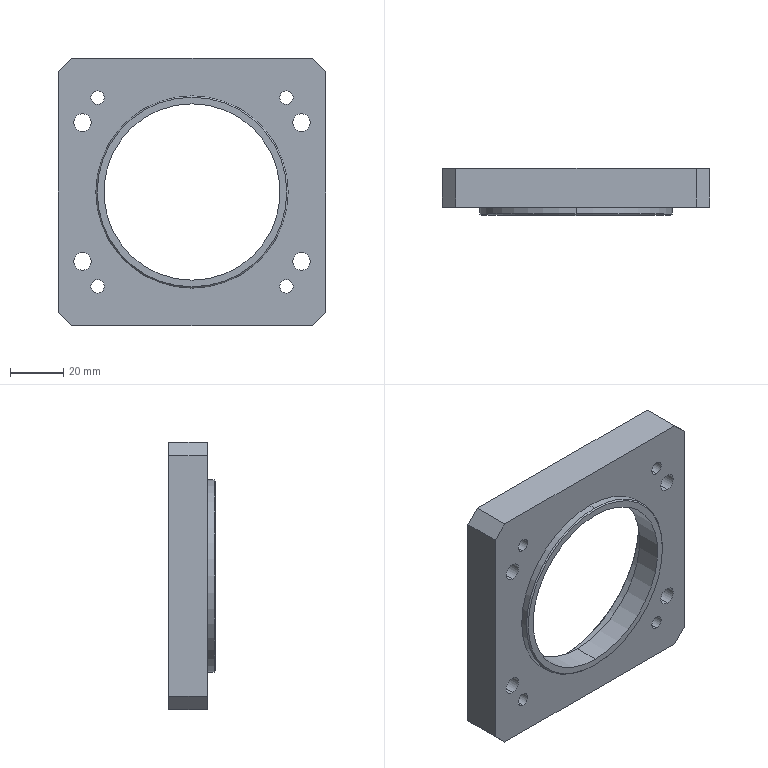Part | SolidWorks | features ICE 6, HoleWzd 4, Chamfer 3, Extrusion 1, Fillet 1 | 1 solid | 50 faces | box 100 x 17.5 x 100 mm | volume 79036 mm3 | cylinder 30 | plane 16 | cone 4 | commonest cylinder face diameters 5 x8 6.6 x8 11 x8 66 x2 72 x2 80 x2
STEP:
#1=CARTESIAN_POINT('',(0.,14.,-40.));
#2=VERTEX_POINT('',#1);
#3=CARTESIAN_POINT('',(0.,14.,40.));
#4=VERTEX_POINT('',#3);
#5=CARTESIAN_POINT('',(0.,14.,0.));
#6=DIRECTION('',(0.,1.,0.));
#7=DIRECTION('',(0.,0.,-1.));
#8=AXIS2_PLACEMENT_3D('',#5,#6,#7);
#9=CIRCLE('',#8,40.);
#10=EDGE_CURVE('',#2,#4,#9,.T.);
#11=ORIENTED_EDGE('',*,*,#10,.F.);
#12=CARTESIAN_POINT('',(0.,14.5,-40.5));
#13=VERTEX_POINT('',#12);
#14=CARTESIAN_POINT('',(0.,14.,-40.));
#15=DIRECTION('',(0.,0.7071,-0.7071));
#16=VECTOR('',#15,1000.);
#17=LINE('',#14,#16);
#18=EDGE_CURVE('',#2,#13,#17,.T.);
#19=ORIENTED_EDGE('',*,*,#18,.T.);
#20=CARTESIAN_POINT('',(0.,14.5,40.5));
#21=VERTEX_POINT('',#20);
#22=CARTESIAN_POINT('',(0.,14.5,0.));
#23=DIRECTION('',(0.,-1.,0.));
#24=DIRECTION('',(0.,0.,-1.));
#25=AXIS2_PLACEMENT_3D('',#22,#23,#24);
#26=CIRCLE('',#25,40.5);
#27=EDGE_CURVE('',#21,#13,#26,.T.);
#28=ORIENTED_EDGE('',*,*,#27,.F.);
#29=CARTESIAN_POINT('',(0.,14.,40.));
#30=DIRECTION('',(0.,0.7071,0.7071));
#31=VECTOR('',#30,1000.);
#32=LINE('',#29,#31);
#33=EDGE_CURVE('',#4,#21,#32,.T.);
#34=ORIENTED_EDGE('',*,*,#33,.F.);
#35=EDGE_LOOP('',(#11,#19,#28,#34));
#36=FACE_OUTER_BOUND('',#35,.T.);
#37=CARTESIAN_POINT('',(0.,14.,0.));
#38=DIRECTION('',(0.,1.,0.));
#39=DIRECTION('',(0.,0.,1.));
#40=AXIS2_PLACEMENT_3D('',#37,#38,#39);
#41=CONICAL_SURFACE('',#40,40.,0.7854);
#42=ADVANCED_FACE('',(#36),#41,.F.);
#43=CARTESIAN_POINT('',(-41.,8.1,-31.5));
#44=VERTEX_POINT('',#43);
#45=CARTESIAN_POINT('',(-41.,8.1,-20.5));
#46=VERTEX_POINT('',#45);
#47=CARTESIAN_POINT('',(-41.,8.1,-26.));
#48=DIRECTION('',(0.,1.,0.));
#49=DIRECTION('',(0.,0.,1.));
#50=AXIS2_PLACEMENT_3D('',#47,#48,#49);
#51=CIRCLE('',#50,5.5);
#52=EDGE_CURVE('',#44,#46,#51,.T.);
#53=ORIENTED_EDGE('',*,*,#52,.F.);
#54=CARTESIAN_POINT('',(-41.,14.5,-31.5));
#55=VERTEX_POINT('',#54);
#56=CARTESIAN_POINT('',(-41.,14.5,-31.5));
#57=DIRECTION('',(0.,1.,0.));
#58=VECTOR('',#57,1000.);
#59=LINE('',#56,#58);
#60=EDGE_CURVE('',#44,#55,#59,.T.);
#61=ORIENTED_EDGE('',*,*,#60,.T.);
#62=CARTESIAN_POINT('',(-41.,14.5,-20.5));
#63=VERTEX_POINT('',#62);
#64=CARTESIAN_POINT('',(-41.,14.5,-26.));
#65=DIRECTION('',(0.,1.,0.));
#66=DIRECTION('',(0.,0.,1.));
#67=AXIS2_PLACEMENT_3D('',#64,#65,#66);
#68=CIRCLE('',#67,5.5);
#69=EDGE_CURVE('',#55,#63,#68,.T.);
#70=ORIENTED_EDGE('',*,*,#69,.T.);
#71=CARTESIAN_POINT('',(-41.,14.5,-20.5));
#72=DIRECTION('',(0.,1.,0.));
#73=VECTOR('',#72,1000.);
#74=LINE('',#71,#73);
#75=EDGE_CURVE('',#46,#63,#74,.T.);
#76=ORIENTED_EDGE('',*,*,#75,.F.);
#77=EDGE_LOOP('',(#53,#61,#70,#76));
#78=FACE_OUTER_BOUND('',#77,.T.);
#79=CARTESIAN_POINT('',(-41.,14.5,-26.));
#80=DIRECTION('',(0.,1.,0.));
#81=DIRECTION('',(0.,0.,1.));
#82=AXIS2_PLACEMENT_3D('',#79,#80,#81);
#83=CYLINDRICAL_SURFACE('',#82,5.5);
#84=ADVANCED_FACE('',(#78),#83,.F.);
#85=CARTESIAN_POINT('',(-41.,0.,-22.7));
#86=VERTEX_POINT('',#85);
#87=CARTESIAN_POINT('',(-41.,0.,-29.3));
#88=VERTEX_POINT('',#87);
#89=CARTESIAN_POINT('',(-41.,0.,-26.));
#90=DIRECTION('',(0.,-1.,0.));
#91=DIRECTION('',(0.,0.,-1.));
#92=AXIS2_PLACEMENT_3D('',#89,#90,#91);
#93=CIRCLE('',#92,3.3);
#94=EDGE_CURVE('',#86,#88,#93,.T.);
#95=ORIENTED_EDGE('',*,*,#94,.T.);
#96=CARTESIAN_POINT('',(-41.,8.1,-29.3));
#97=VERTEX_POINT('',#96);
#98=CARTESIAN_POINT('',(-41.,14.5,-29.3));
#99=DIRECTION('',(0.,1.,0.));
#100=VECTOR('',#99,1000.);
#101=LINE('',#98,#100);
#102=EDGE_CURVE('',#88,#97,#101,.T.);
#103=ORIENTED_EDGE('',*,*,#102,.T.);
#104=CARTESIAN_POINT('',(-41.,8.1,-22.7));
#105=VERTEX_POINT('',#104);
#106=CARTESIAN_POINT('',(-41.,8.1,-26.));
#107=DIRECTION('',(0.,1.,0.));
#108=DIRECTION('',(0.,0.,1.));
#109=AXIS2_PLACEMENT_3D('',#106,#107,#108);
#110=CIRCLE('',#109,3.3);
#111=EDGE_CURVE('',#97,#105,#110,.T.);
#112=ORIENTED_EDGE('',*,*,#111,.T.);
#113=CARTESIAN_POINT('',(-41.,14.5,-22.7));
#114=DIRECTION('',(0.,1.,0.));
#115=VECTOR('',#114,1000.);
#116=LINE('',#113,#115);
#117=EDGE_CURVE('',#86,#105,#116,.T.);
#118=ORIENTED_EDGE('',*,*,#117,.F.);
#119=EDGE_LOOP('',(#95,#103,#112,#118));
#120=FACE_OUTER_BOUND('',#119,.T.);
#121=CARTESIAN_POINT('',(-41.,14.5,-26.));
#122=DIRECTION('',(0.,1.,0.));
#123=DIRECTION('',(0.,0.,1.));
#124=AXIS2_PLACEMENT_3D('',#121,#122,#123);
#125=CYLINDRICAL_SURFACE('',#124,3.3);
#126=ADVANCED_FACE('',(#120),#125,.F.);
#127=CARTESIAN_POINT('',(41.,8.1,20.5));
#128=VERTEX_POINT('',#127);
#129=CARTESIAN_POINT('',(41.,8.1,31.5));
#130=VERTEX_POINT('',#129);
#131=CARTESIAN_POINT('',(41.,8.1,26.));
#132=DIRECTION('',(0.,1.,0.));
#133=DIRECTION('',(0.,0.,1.));
#134=AXIS2_PLACEMENT_3D('',#131,#132,#133);
#135=CIRCLE('',#134,5.5);
#136=EDGE_CURVE('',#128,#130,#135,.T.);
#137=ORIENTED_EDGE('',*,*,#136,.F.);
#138=CARTESIAN_POINT('',(41.,14.5,20.5));
#139=VERTEX_POINT('',#138);
#140=CARTESIAN_POINT('',(41.,14.5,20.5));
#141=DIRECTION('',(0.,1.,0.));
#142=VECTOR('',#141,1000.);
#143=LINE('',#140,#142);
#144=EDGE_CURVE('',#128,#139,#143,.T.);
#145=ORIENTED_EDGE('',*,*,#144,.T.);
#146=CARTESIAN_POINT('',(41.,14.5,31.5));
#147=VERTEX_POINT('',#146);
#148=CARTESIAN_POINT('',(41.,14.5,26.));
#149=DIRECTION('',(0.,1.,0.));
#150=DIRECTION('',(0.,0.,1.));
#151=AXIS2_PLACEMENT_3D('',#148,#149,#150);
#152=CIRCLE('',#151,5.5);
#153=EDGE_CURVE('',#139,#147,#152,.T.);
#154=ORIENTED_EDGE('',*,*,#153,.T.);
#155=CARTESIAN_POINT('',(41.,14.5,31.5));
#156=DIRECTION('',(0.,1.,0.));
#157=VECTOR('',#156,1000.);
#158=LINE('',#155,#157);
#159=EDGE_CURVE('',#130,#147,#158,.T.);
#160=ORIENTED_EDGE('',*,*,#159,.F.);
#161=EDGE_LOOP('',(#137,#145,#154,#160));
#162=FACE_OUTER_BOUND('',#161,.T.);
#163=CARTESIAN_POINT('',(41.,14.5,26.));
#164=DIRECTION('',(0.,1.,0.));
#165=DIRECTION('',(0.,0.,1.));
#166=AXIS2_PLACEMENT_3D('',#163,#164,#165);
#167=CYLINDRICAL_SURFACE('',#166,5.5);
#168=ADVANCED_FACE('',(#162),#167,.F.);
#169=CARTESIAN_POINT('',(41.,0.,29.3));
#170=VERTEX_POINT('',#169);
#171=CARTESIAN_POINT('',(41.,0.,22.7));
#172=VERTEX_POINT('',#171);
#173=CARTESIAN_POINT('',(41.,0.,26.));
#174=DIRECTION('',(0.,-1.,0.));
#175=DIRECTION('',(0.,0.,-1.));
#176=AXIS2_PLACEMENT_3D('',#173,#174,#175);
#177=CIRCLE('',#176,3.3);
#178=EDGE_CURVE('',#170,#172,#177,.T.);
#179=ORIENTED_EDGE('',*,*,#178,.T.);
#180=CARTESIAN_POINT('',(41.,8.1,22.7));
#181=VERTEX_POINT('',#180);
#182=CARTESIAN_POINT('',(41.,14.5,22.7));
#183=DIRECTION('',(0.,1.,0.));
#184=VECTOR('',#183,1000.);
#185=LINE('',#182,#184);
#186=EDGE_CURVE('',#172,#181,#185,.T.);
#187=ORIENTED_EDGE('',*,*,#186,.T.);
#188=CARTESIAN_POINT('',(41.,8.1,29.3));
#189=VERTEX_POINT('',#188);
#190=CARTESIAN_POINT('',(41.,8.1,26.));
#191=DIRECTION('',(0.,1.,0.));
#192=DIRECTION('',(0.,0.,1.));
#193=AXIS2_PLACEMENT_3D('',#190,#191,#192);
#194=CIRCLE('',#193,3.3);
#195=EDGE_CURVE('',#181,#189,#194,.T.);
#196=ORIENTED_EDGE('',*,*,#195,.T.);
#197=CARTESIAN_POINT('',(41.,14.5,29.3));
#198=DIRECTION('',(0.,1.,0.));
#199=VECTOR('',#198,1000.);
#200=LINE('',#197,#199);
#201=EDGE_CURVE('',#170,#189,#200,.T.);
#202=ORIENTED_EDGE('',*,*,#201,.F.);
#203=EDGE_LOOP('',(#179,#187,#196,#202));
#204=FACE_OUTER_BOUND('',#203,.T.);
#205=CARTESIAN_POINT('',(41.,14.5,26.));
#206=DIRECTION('',(0.,1.,0.));
#207=DIRECTION('',(0.,0.,1.));
#208=AXIS2_PLACEMENT_3D('',#205,#206,#207);
#209=CYLINDRICAL_SURFACE('',#208,3.3);
#210=ADVANCED_FACE('',(#204),#209,.F.);
#211=CARTESIAN_POINT('',(41.,8.1,-31.5));
#212=VERTEX_POINT('',#211);
#213=CARTESIAN_POINT('',(41.,8.1,-20.5));
#214=VERTEX_POINT('',#213);
#215=CARTESIAN_POINT('',(41.,8.1,-26.));
#216=DIRECTION('',(0.,1.,0.));
#217=DIRECTION('',(0.,0.,1.));
#218=AXIS2_PLACEMENT_3D('',#215,#216,#217);
#219=CIRCLE('',#218,5.5);
#220=EDGE_CURVE('',#212,#214,#219,.T.);
#221=ORIENTED_EDGE('',*,*,#220,.F.);
#222=CARTESIAN_POINT('',(41.,14.5,-31.5));
#223=VERTEX_POINT('',#222);
#224=CARTESIAN_POINT('',(41.,14.5,-31.5));
#225=DIRECTION('',(0.,1.,0.));
#226=VECTOR('',#225,1000.);
#227=LINE('',#224,#226);
#228=EDGE_CURVE('',#212,#223,#227,.T.);
#229=ORIENTED_EDGE('',*,*,#228,.T.);
#230=CARTESIAN_POINT('',(41.,14.5,-20.5));
#231=VERTEX_POINT('',#230);
#232=CARTESIAN_POINT('',(41.,14.5,-26.));
#233=DIRECTION('',(0.,1.,0.));
#234=DIRECTION('',(0.,0.,1.));
#235=AXIS2_PLACEMENT_3D('',#232,#233,#234);
#236=CIRCLE('',#235,5.5);
#237=EDGE_CURVE('',#223,#231,#236,.T.);
#238=ORIENTED_EDGE('',*,*,#237,.T.);
#239=CARTESIAN_POINT('',(41.,14.5,-20.5));
#240=DIRECTION('',(0.,1.,0.));
#241=VECTOR('',#240,1000.);
#242=LINE('',#239,#241);
#243=EDGE_CURVE('',#214,#231,#242,.T.);
#244=ORIENTED_EDGE('',*,*,#243,.F.);
#245=EDGE_LOOP('',(#221,#229,#238,#244));
#246=FACE_OUTER_BOUND('',#245,.T.);
#247=CARTESIAN_POINT('',(41.,14.5,-26.));
#248=DIRECTION('',(0.,1.,0.));
#249=DIRECTION('',(0.,0.,1.));
#250=AXIS2_PLACEMENT_3D('',#247,#248,#249);
#251=CYLINDRICAL_SURFACE('',#250,5.5);
#252=ADVANCED_FACE('',(#246),#251,.F.);
#253=CARTESIAN_POINT('',(41.,0.,-22.7));
#254=VERTEX_POINT('',#253);
#255=CARTESIAN_POINT('',(41.,0.,-29.3));
#256=VERTEX_POINT('',#255);
#257=CARTESIAN_POINT('',(41.,0.,-26.));
#258=DIRECTION('',(0.,-1.,0.));
#259=DIRECTION('',(0.,0.,-1.));
#260=AXIS2_PLACEMENT_3D('',#257,#258,#259);
#261=CIRCLE('',#260,3.3);
#262=EDGE_CURVE('',#254,#256,#261,.T.);
#263=ORIENTED_EDGE('',*,*,#262,.T.);
#264=CARTESIAN_POINT('',(41.,8.1,-29.3));
#265=VERTEX_POINT('',#264);
#266=CARTESIAN_POINT('',(41.,14.5,-29.3));
#267=DIRECTION('',(0.,1.,0.));
#268=VECTOR('',#267,1000.);
#269=LINE('',#266,#268);
#270=EDGE_CURVE('',#256,#265,#269,.T.);
#271=ORIENTED_EDGE('',*,*,#270,.T.);
#272=CARTESIAN_POINT('',(41.,8.1,-22.7));
#273=VERTEX_POINT('',#272);
#274=CARTESIAN_POINT('',(41.,8.1,-26.));
#275=DIRECTION('',(0.,1.,0.));
#276=DIRECTION('',(0.,0.,1.));
#277=AXIS2_PLACEMENT_3D('',#274,#275,#276);
#278=CIRCLE('',#277,3.3);
#279=EDGE_CURVE('',#265,#273,#278,.T.);
#280=ORIENTED_EDGE('',*,*,#279,.T.);
#281=CARTESIAN_POINT('',(41.,14.5,-22.7));
#282=DIRECTION('',(0.,1.,0.));
#283=VECTOR('',#282,1000.);
#284=LINE('',#281,#283);
#285=EDGE_CURVE('',#254,#273,#284,.T.);
#286=ORIENTED_EDGE('',*,*,#285,.F.);
#287=EDGE_LOOP('',(#263,#271,#280,#286));
#288=FACE_OUTER_BOUND('',#287,.T.);
#289=CARTESIAN_POINT('',(41.,14.5,-26.));
#290=DIRECTION('',(0.,1.,0.));
#291=DIRECTION('',(0.,0.,1.));
#292=AXIS2_PLACEMENT_3D('',#289,#290,#291);
#293=CYLINDRICAL_SURFACE('',#292,3.3);
#294=ADVANCED_FACE('',(#288),#293,.F.);
#295=CARTESIAN_POINT('',(-41.,8.1,20.5));
#296=VERTEX_POINT('',#295);
#297=CARTESIAN_POINT('',(-41.,8.1,31.5));
#298=VERTEX_POINT('',#297);
#299=CARTESIAN_POINT('',(-41.,8.1,26.));
#300=DIRECTION('',(0.,1.,0.));
#301=DIRECTION('',(0.,0.,1.));
#302=AXIS2_PLACEMENT_3D('',#299,#300,#301);
#303=CIRCLE('',#302,5.5);
#304=EDGE_CURVE('',#296,#298,#303,.T.);
#305=ORIENTED_EDGE('',*,*,#304,.F.);
#306=CARTESIAN_POINT('',(-41.,14.5,20.5));
#307=VERTEX_POINT('',#306);
#308=CARTESIAN_POINT('',(-41.,14.5,20.5));
#309=DIRECTION('',(0.,1.,0.));
#310=VECTOR('',#309,1000.);
#311=LINE('',#308,#310);
#312=EDGE_CURVE('',#296,#307,#311,.T.);
#313=ORIENTED_EDGE('',*,*,#312,.T.);
#314=CARTESIAN_POINT('',(-41.,14.5,31.5));
#315=VERTEX_POINT('',#314);
#316=CARTESIAN_POINT('',(-41.,14.5,26.));
#317=DIRECTION('',(0.,1.,0.));
#318=DIRECTION('',(0.,0.,1.));
#319=AXIS2_PLACEMENT_3D('',#316,#317,#318);
#320=CIRCLE('',#319,5.5);
#321=EDGE_CURVE('',#307,#315,#320,.T.);
#322=ORIENTED_EDGE('',*,*,#321,.T.);
#323=CARTESIAN_POINT('',(-41.,14.5,31.5));
#324=DIRECTION('',(0.,1.,0.));
#325=VECTOR('',#324,1000.);
#326=LINE('',#323,#325);
#327=EDGE_CURVE('',#298,#315,#326,.T.);
#328=ORIENTED_EDGE('',*,*,#327,.F.);
#329=EDGE_LOOP('',(#305,#313,#322,#328));
#330=FACE_OUTER_BOUND('',#329,.T.);
#331=CARTESIAN_POINT('',(-41.,14.5,26.));
#332=DIRECTION('',(0.,1.,0.));
#333=DIRECTION('',(0.,0.,1.));
#334=AXIS2_PLACEMENT_3D('',#331,#332,#333);
#335=CYLINDRICAL_SURFACE('',#334,5.5);
#336=ADVANCED_FACE('',(#330),#335,.F.);
#337=CARTESIAN_POINT('',(-41.,0.,29.3));
#338=VERTEX_POINT('',#337);
#339=CARTESIAN_POINT('',(-41.,0.,22.7));
#340=VERTEX_POINT('',#339);
#341=CARTESIAN_POINT('',(-41.,0.,26.));
#342=DIRECTION('',(0.,-1.,0.));
#343=DIRECTION('',(0.,0.,-1.));
#344=AXIS2_PLACEMENT_3D('',#341,#342,#343);
#345=CIRCLE('',#344,3.3);
#346=EDGE_CURVE('',#338,#340,#345,.T.);
#347=ORIENTED_EDGE('',*,*,#346,.T.);
#348=CARTESIAN_POINT('',(-41.,8.1,22.7));
#349=VERTEX_POINT('',#348);
#350=CARTESIAN_POINT('',(-41.,14.5,22.7));
#351=DIRECTION('',(0.,1.,0.));
#352=VECTOR('',#351,1000.);
#353=LINE('',#350,#352);
#354=EDGE_CURVE('',#340,#349,#353,.T.);
#355=ORIENTED_EDGE('',*,*,#354,.T.);
#356=CARTESIAN_POINT('',(-41.,8.1,29.3));
#357=VERTEX_POINT('',#356);
#358=CARTESIAN_POINT('',(-41.,8.1,26.));
#359=DIRECTION('',(0.,1.,0.));
#360=DIRECTION('',(0.,0.,1.));
#361=AXIS2_PLACEMENT_3D('',#358,#359,#360);
#362=CIRCLE('',#361,3.3);
#363=EDGE_CURVE('',#349,#357,#362,.T.);
#364=ORIENTED_EDGE('',*,*,#363,.T.);
#365=CARTESIAN_POINT('',(-41.,14.5,29.3));
#366=DIRECTION('',(0.,1.,0.));
#367=VECTOR('',#366,1000.);
#368=LINE('',#365,#367);
#369=EDGE_CURVE('',#338,#357,#368,.T.);
#370=ORIENTED_EDGE('',*,*,#369,.F.);
#371=EDGE_LOOP('',(#347,#355,#364,#370));
#372=FACE_OUTER_BOUND('',#371,.T.);
#373=CARTESIAN_POINT('',(-41.,14.5,26.));
#374=DIRECTION('',(0.,1.,0.));
#375=DIRECTION('',(0.,0.,1.));
#376=AXIS2_PLACEMENT_3D('',#373,#374,#375);
#377=CYLINDRICAL_SURFACE('',#376,3.3);
#378=ADVANCED_FACE('',(#372),#377,.F.);
#379=CARTESIAN_POINT('',(-35.355,0.,-32.855));
#380=VERTEX_POINT('',#379);
#381=CARTESIAN_POINT('',(-35.355,0.,-37.855));
#382=VERTEX_POINT('',#381);
#383=CARTESIAN_POINT('',(-35.355,0.,-35.355));
#384=DIRECTION('',(0.,-1.,0.));
#385=DIRECTION('',(0.,0.,-1.));
#386=AXIS2_PLACEMENT_3D('',#383,#384,#385);
#387=CIRCLE('',#386,2.5);
#388=EDGE_CURVE('',#380,#382,#387,.T.);
#389=ORIENTED_EDGE('',*,*,#388,.T.);
#390=CARTESIAN_POINT('',(-35.355,14.5,-37.855));
#391=VERTEX_POINT('',#390);
#392=CARTESIAN_POINT('',(-35.355,14.5,-37.855));
#393=DIRECTION('',(0.,1.,0.));
#394=VECTOR('',#393,1000.);
#395=LINE('',#392,#394);
#396=EDGE_CURVE('',#382,#391,#395,.T.);
#397=ORIENTED_EDGE('',*,*,#396,.T.);
#398=CARTESIAN_POINT('',(-35.355,14.5,-32.855));
#399=VERTEX_POINT('',#398);
#400=CARTESIAN_POINT('',(-35.355,14.5,-35.355));
#401=DIRECTION('',(0.,1.,0.));
#402=DIRECTION('',(0.,0.,1.));
#403=AXIS2_PLACEMENT_3D('',#400,#401,#402);
#404=CIRCLE('',#403,2.5);
#405=EDGE_CURVE('',#391,#399,#404,.T.);
#406=ORIENTED_EDGE('',*,*,#405,.T.);
#407=CARTESIAN_POINT('',(-35.355,14.5,-32.855));
#408=DIRECTION('',(0.,1.,0.));
#409=VECTOR('',#408,1000.);
#410=LINE('',#407,#409);
#411=EDGE_CURVE('',#380,#399,#410,.T.);
#412=ORIENTED_EDGE('',*,*,#411,.F.);
#413=EDGE_LOOP('',(#389,#397,#406,#412));
#414=FACE_OUTER_BOUND('',#413,.T.);
#415=CARTESIAN_POINT('',(-35.355,14.5,-35.355));
#416=DIRECTION('',(0.,1.,0.));
#417=DIRECTION('',(0.,0.,1.));
#418=AXIS2_PLACEMENT_3D('',#415,#416,#417);
#419=CYLINDRICAL_SURFACE('',#418,2.5);
#420=ADVANCED_FACE('',(#414),#419,.F.);
#421=CARTESIAN_POINT('',(35.355,0.,-32.855));
#422=VERTEX_POINT('',#421);
#423=CARTESIAN_POINT('',(35.355,0.,-37.855));
#424=VERTEX_POINT('',#423);
#425=CARTESIAN_POINT('',(35.355,0.,-35.355));
#426=DIRECTION('',(0.,-1.,0.));
#427=DIRECTION('',(0.,0.,-1.));
#428=AXIS2_PLACEMENT_3D('',#425,#426,#427);
#429=CIRCLE('',#428,2.5);
#430=EDGE_CURVE('',#422,#424,#429,.T.);
#431=ORIENTED_EDGE('',*,*,#430,.T.);
#432=CARTESIAN_POINT('',(35.355,14.5,-37.855));
#433=VERTEX_POINT('',#432);
#434=CARTESIAN_POINT('',(35.355,14.5,-37.855));
#435=DIRECTION('',(0.,1.,0.));
#436=VECTOR('',#435,1000.);
#437=LINE('',#434,#436);
#438=EDGE_CURVE('',#424,#433,#437,.T.);
#439=ORIENTED_EDGE('',*,*,#438,.T.);
#440=CARTESIAN_POINT('',(35.355,14.5,-32.855));
#441=VERTEX_POINT('',#440);
#442=CARTESIAN_POINT('',(35.355,14.5,-35.355));
#443=DIRECTION('',(0.,1.,0.));
#444=DIRECTION('',(0.,0.,1.));
#445=AXIS2_PLACEMENT_3D('',#442,#443,#444);
#446=CIRCLE('',#445,2.5);
#447=EDGE_CURVE('',#433,#441,#446,.T.);
#448=ORIENTED_EDGE('',*,*,#447,.T.);
#449=CARTESIAN_POINT('',(35.355,14.5,-32.855));
#450=DIRECTION('',(0.,1.,0.));
#451=VECTOR('',#450,1000.);
#452=LINE('',#449,#451);
#453=EDGE_CURVE('',#422,#441,#452,.T.);
#454=ORIENTED_EDGE('',*,*,#453,.F.);
#455=EDGE_LOOP('',(#431,#439,#448,#454));
#456=FACE_OUTER_BOUND('',#455,.T.);
#457=CARTESIAN_POINT('',(35.355,14.5,-35.355));
#458=DIRECTION('',(0.,1.,0.));
#459=DIRECTION('',(0.,0.,1.));
#460=AXIS2_PLACEMENT_3D('',#457,#458,#459);
#461=CYLINDRICAL_SURFACE('',#460,2.5);
#462=ADVANCED_FACE('',(#456),#461,.F.);
#463=CARTESIAN_POINT('',(-35.355,0.,37.855));
#464=VERTEX_POINT('',#463);
#465=CARTESIAN_POINT('',(-35.355,0.,32.855));
#466=VERTEX_POINT('',#465);
#467=CARTESIAN_POINT('',(-35.355,0.,35.355));
#468=DIRECTION('',(0.,-1.,0.));
#469=DIRECTION('',(0.,0.,-1.));
#470=AXIS2_PLACEMENT_3D('',#467,#468,#469);
#471=CIRCLE('',#470,2.5);
#472=EDGE_CURVE('',#464,#466,#471,.T.);
#473=ORIENTED_EDGE('',*,*,#472,.T.);
#474=CARTESIAN_POINT('',(-35.355,14.5,32.855));
#475=VERTEX_POINT('',#474);
#476=CARTESIAN_POINT('',(-35.355,14.5,32.855));
#477=DIRECTION('',(0.,1.,0.));
#478=VECTOR('',#477,1000.);
#479=LINE('',#476,#478);
#480=EDGE_CURVE('',#466,#475,#479,.T.);
#481=ORIENTED_EDGE('',*,*,#480,.T.);
#482=CARTESIAN_POINT('',(-35.355,14.5,37.855));
#483=VERTEX_POINT('',#482);
#484=CARTESIAN_POINT('',(-35.355,14.5,35.355));
#485=DIRECTION('',(0.,1.,0.));
#486=DIRECTION('',(0.,0.,1.));
#487=AXIS2_PLACEMENT_3D('',#484,#485,#486);
#488=CIRCLE('',#487,2.5);
#489=EDGE_CURVE('',#475,#483,#488,.T.);
#490=ORIENTED_EDGE('',*,*,#489,.T.);
#491=CARTESIAN_POINT('',(-35.355,14.5,37.855));
#492=DIRECTION('',(0.,1.,0.));
#493=VECTOR('',#492,1000.);
#494=LINE('',#491,#493);
#495=EDGE_CURVE('',#464,#483,#494,.T.);
#496=ORIENTED_EDGE('',*,*,#495,.F.);
#497=EDGE_LOOP('',(#473,#481,#490,#496));
#498=FACE_OUTER_BOUND('',#497,.T.);
#499=CARTESIAN_POINT('',(-35.355,14.5,35.355));
#500=DIRECTION('',(0.,1.,0.));
#501=DIRECTION('',(0.,0.,1.));
#502=AXIS2_PLACEMENT_3D('',#499,#500,#501);
#503=CYLINDRICAL_SURFACE('',#502,2.5);
#504=ADVANCED_FACE('',(#498),#503,.F.);
#505=CARTESIAN_POINT('',(35.355,0.,37.855));
#506=VERTEX_POINT('',#505);
#507=CARTESIAN_POINT('',(35.355,0.,32.855));
#508=VERTEX_POINT('',#507);
#509=CARTESIAN_POINT('',(35.355,0.,35.355));
#510=DIRECTION('',(0.,-1.,0.));
#511=DIRECTION('',(0.,0.,-1.));
#512=AXIS2_PLACEMENT_3D('',#509,#510,#511);
#513=CIRCLE('',#512,2.5);
#514=EDGE_CURVE('',#506,#508,#513,.T.);
#515=ORIENTED_EDGE('',*,*,#514,.T.);
#516=CARTESIAN_POINT('',(35.355,14.5,32.855));
#517=VERTEX_POINT('',#516);
#518=CARTESIAN_POINT('',(35.355,14.5,32.855));
#519=DIRECTION('',(0.,1.,0.));
#520=VECTOR('',#519,1000.);
#521=LINE('',#518,#520);
#522=EDGE_CURVE('',#508,#517,#521,.T.);
#523=ORIENTED_EDGE('',*,*,#522,.T.);
#524=CARTESIAN_POINT('',(35.355,14.5,37.855));
#525=VERTEX_POINT('',#524);
#526=CARTESIAN_POINT('',(35.355,14.5,35.355));
#527=DIRECTION('',(0.,1.,0.));
#528=DIRECTION('',(0.,0.,1.));
#529=AXIS2_PLACEMENT_3D('',#526,#527,#528);
#530=CIRCLE('',#529,2.5);
#531=EDGE_CURVE('',#517,#525,#530,.T.);
#532=ORIENTED_EDGE('',*,*,#531,.T.);
#533=CARTESIAN_POINT('',(35.355,14.5,37.855));
#534=DIRECTION('',(0.,1.,0.));
#535=VECTOR('',#534,1000.);
#536=LINE('',#533,#535);
#537=EDGE_CURVE('',#506,#525,#536,.T.);
#538=ORIENTED_EDGE('',*,*,#537,.F.);
#539=EDGE_LOOP('',(#515,#523,#532,#538));
#540=FACE_OUTER_BOUND('',#539,.T.);
#541=CARTESIAN_POINT('',(35.355,14.5,35.355));
#542=DIRECTION('',(0.,1.,0.));
#543=DIRECTION('',(0.,0.,1.));
#544=AXIS2_PLACEMENT_3D('',#541,#542,#543);
#545=CYLINDRICAL_SURFACE('',#544,2.5);
#546=ADVANCED_FACE('',(#540),#545,.F.);
#547=CARTESIAN_POINT('',(0.,6.5,-40.));
#548=VERTEX_POINT('',#547);
#549=CARTESIAN_POINT('',(0.,6.5,40.));
#550=VERTEX_POINT('',#549);
#551=CARTESIAN_POINT('',(0.,6.5,0.));
#552=DIRECTION('',(0.,1.,0.));
#553=DIRECTION('',(0.,0.,1.));
#554=AXIS2_PLACEMENT_3D('',#551,#552,#553);
#555=CIRCLE('',#554,40.);
#556=EDGE_CURVE('',#548,#550,#555,.T.);
#557=ORIENTED_EDGE('',*,*,#556,.F.);
#558=CARTESIAN_POINT('',(0.,6.5,-40.));
#559=DIRECTION('',(0.,1.,0.));
#560=VECTOR('',#559,1000.);
#561=LINE('',#558,#560);
#562=EDGE_CURVE('',#548,#2,#561,.T.);
#563=ORIENTED_EDGE('',*,*,#562,.T.);
#564=ORIENTED_EDGE('',*,*,#10,.T.);
#565=CARTESIAN_POINT('',(0.,6.5,40.));
#566=DIRECTION('',(0.,1.,0.));
#567=VECTOR('',#566,1000.);
#568=LINE('',#565,#567);
#569=EDGE_CURVE('',#550,#4,#568,.T.);
#570=ORIENTED_EDGE('',*,*,#569,.F.);
#571=EDGE_LOOP('',(#557,#563,#564,#570));
#572=FACE_OUTER_BOUND('',#571,.T.);
#573=CARTESIAN_POINT('',(0.,6.5,0.));
#574=DIRECTION('',(0.,1.,0.));
#575=DIRECTION('',(0.,0.,1.));
#576=AXIS2_PLACEMENT_3D('',#573,#574,#575);
#577=CYLINDRICAL_SURFACE('',#576,40.);
#578=ADVANCED_FACE('',(#572),#577,.F.);
#579=CARTESIAN_POINT('',(0.,-3.,-35.5));
#580=VERTEX_POINT('',#579);
#581=CARTESIAN_POINT('',(0.,-3.,35.5));
#582=VERTEX_POINT('',#581);
#583=CARTESIAN_POINT('',(0.,-3.,0.));
#584=DIRECTION('',(0.,-1.,0.));
#585=DIRECTION('',(0.,0.,-1.));
#586=AXIS2_PLACEMENT_3D('',#583,#584,#585);
#587=CIRCLE('',#586,35.5);
#588=EDGE_CURVE('',#580,#582,#587,.T.);
#589=ORIENTED_EDGE('',*,*,#588,.F.);
#590=CARTESIAN_POINT('',(0.,-2.5,-36.));
#591=VERTEX_POINT('',#590);
#592=CARTESIAN_POINT('',(0.,-3.,-35.5));
#593=DIRECTION('',(0.,0.7071,-0.7071));
#594=VECTOR('',#593,1000.);
#595=LINE('',#592,#594);
#596=EDGE_CURVE('',#580,#591,#595,.T.);
#597=ORIENTED_EDGE('',*,*,#596,.T.);
#598=CARTESIAN_POINT('',(0.,-2.5,36.));
#599=VERTEX_POINT('',#598);
#600=CARTESIAN_POINT('',(0.,-2.5,0.));
#601=DIRECTION('',(0.,1.,0.));
#602=DIRECTION('',(0.,0.,-1.));
#603=AXIS2_PLACEMENT_3D('',#600,#601,#602);
#604=CIRCLE('',#603,36.);
#605=EDGE_CURVE('',#599,#591,#604,.T.);
#606=ORIENTED_EDGE('',*,*,#605,.F.);
#607=CARTESIAN_POINT('',(0.,-3.,35.5));
#608=DIRECTION('',(0.,0.7071,0.7071));
#609=VECTOR('',#608,1000.);
#610=LINE('',#607,#609);
#611=EDGE_CURVE('',#582,#599,#610,.T.);
#612=ORIENTED_EDGE('',*,*,#611,.F.);
#613=EDGE_LOOP('',(#589,#597,#606,#612));
#614=FACE_OUTER_BOUND('',#613,.T.);
#615=CARTESIAN_POINT('',(0.,-3.,0.));
#616=DIRECTION('',(0.,1.,0.));
#617=DIRECTION('',(0.,0.,1.));
#618=AXIS2_PLACEMENT_3D('',#615,#616,#617);
#619=CONICAL_SURFACE('',#618,35.5,0.7854);
#620=ADVANCED_FACE('',(#614),#619,.T.);
#621=ORIENTED_EDGE('',*,*,#605,.T.);
#622=CARTESIAN_POINT('',(0.,0.,-36.));
#623=VERTEX_POINT('',#622);
#624=CARTESIAN_POINT('',(0.,-3.,-36.));
#625=DIRECTION('',(0.,1.,0.));
#626=VECTOR('',#625,1000.);
#627=LINE('',#624,#626);
#628=EDGE_CURVE('',#591,#623,#627,.T.);
#629=ORIENTED_EDGE('',*,*,#628,.T.);
#630=CARTESIAN_POINT('',(0.,0.,36.));
#631=VERTEX_POINT('',#630);
#632=CARTESIAN_POINT('',(0.,0.,0.));
#633=DIRECTION('',(0.,-1.,0.));
#634=DIRECTION('',(0.,0.,-1.));
#635=AXIS2_PLACEMENT_3D('',#632,#633,#634);
#636=CIRCLE('',#635,36.);
#637=EDGE_CURVE('',#623,#631,#636,.T.);
#638=ORIENTED_EDGE('',*,*,#637,.T.);
#639=CARTESIAN_POINT('',(0.,-3.,36.));
#640=DIRECTION('',(0.,1.,0.));
#641=VECTOR('',#640,1000.);
#642=LINE('',#639,#641);
#643=EDGE_CURVE('',#599,#631,#642,.T.);
#644=ORIENTED_EDGE('',*,*,#643,.F.);
#645=EDGE_LOOP('',(#621,#629,#638,#644));
#646=FACE_OUTER_BOUND('',#645,.T.);
#647=CARTESIAN_POINT('',(0.,-3.,0.));
#648=DIRECTION('',(0.,1.,0.));
#649=DIRECTION('',(0.,0.,1.));
#650=AXIS2_PLACEMENT_3D('',#647,#648,#649);
#651=CYLINDRICAL_SURFACE('',#650,36.);
#652=ADVANCED_FACE('',(#646),#651,.T.);
#653=CARTESIAN_POINT('',(0.,-3.,33.));
#654=VERTEX_POINT('',#653);
#655=CARTESIAN_POINT('',(0.,-3.,-33.));
#656=VERTEX_POINT('',#655);
#657=CARTESIAN_POINT('',(0.,-3.,0.));
#658=DIRECTION('',(0.,-1.,0.));
#659=DIRECTION('',(0.,0.,-1.));
#660=AXIS2_PLACEMENT_3D('',#657,#658,#659);
#661=CIRCLE('',#660,33.);
#662=EDGE_CURVE('',#654,#656,#661,.T.);
#663=ORIENTED_EDGE('',*,*,#662,.T.);
#664=CARTESIAN_POINT('',(0.,6.5,-33.));
#665=VERTEX_POINT('',#664);
#666=CARTESIAN_POINT('',(0.,-3.,-33.));
#667=DIRECTION('',(0.,1.,0.));
#668=VECTOR('',#667,1000.);
#669=LINE('',#666,#668);
#670=EDGE_CURVE('',#656,#665,#669,.T.);
#671=ORIENTED_EDGE('',*,*,#670,.T.);
#672=CARTESIAN_POINT('',(0.,6.5,33.));
#673=VERTEX_POINT('',#672);
#674=CARTESIAN_POINT('',(0.,6.5,0.));
#675=DIRECTION('',(0.,1.,0.));
#676=DIRECTION('',(0.,0.,1.));
#677=AXIS2_PLACEMENT_3D('',#674,#675,#676);
#678=CIRCLE('',#677,33.);
#679=EDGE_CURVE('',#665,#673,#678,.T.);
#680=ORIENTED_EDGE('',*,*,#679,.T.);
#681=CARTESIAN_POINT('',(0.,-3.,33.));
#682=DIRECTION('',(0.,1.,0.));
#683=VECTOR('',#682,1000.);
#684=LINE('',#681,#683);
#685=EDGE_CURVE('',#654,#673,#684,.T.);
#686=ORIENTED_EDGE('',*,*,#685,.F.);
#687=EDGE_LOOP('',(#663,#671,#680,#686));
#688=FACE_OUTER_BOUND('',#687,.T.);
#689=CARTESIAN_POINT('',(0.,-3.,0.));
#690=DIRECTION('',(0.,1.,0.));
#691=DIRECTION('',(0.,0.,1.));
#692=AXIS2_PLACEMENT_3D('',#689,#690,#691);
#693=CYLINDRICAL_SURFACE('',#692,33.);
#694=ADVANCED_FACE('',(#688),#693,.F.);
#695=ORIENTED_EDGE('',*,*,#670,.F.);
#696=CARTESIAN_POINT('',(0.,-3.,0.));
#697=DIRECTION('',(0.,-1.,0.));
#698=DIRECTION('',(0.,0.,-1.));
#699=AXIS2_PLACEMENT_3D('',#696,#697,#698);
#700=CIRCLE('',#699,33.);
#701=EDGE_CURVE('',#656,#654,#700,.T.);
#702=ORIENTED_EDGE('',*,*,#701,.T.);
#703=ORIENTED_EDGE('',*,*,#685,.T.);
#704=CARTESIAN_POINT('',(0.,6.5,0.));
#705=DIRECTION('',(0.,1.,0.));
#706=DIRECTION('',(0.,0.,1.));
#707=AXIS2_PLACEMENT_3D('',#704,#705,#706);
#708=CIRCLE('',#707,33.);
#709=EDGE_CURVE('',#673,#665,#708,.T.);
#710=ORIENTED_EDGE('',*,*,#709,.T.);
#711=EDGE_LOOP('',(#695,#702,#703,#710));
#712=FACE_OUTER_BOUND('',#711,.T.);
#713=CARTESIAN_POINT('',(0.,-3.,0.));
#714=DIRECTION('',(0.,1.,0.));
#715=DIRECTION('',(0.,0.,1.));
#716=AXIS2_PLACEMENT_3D('',#713,#714,#715);
#717=CYLINDRICAL_SURFACE('',#716,33.);
#718=ADVANCED_FACE('',(#712),#717,.F.);
#719=CARTESIAN_POINT('',(50.,14.5,45.));
#720=VERTEX_POINT('',#719);
#721=CARTESIAN_POINT('',(50.,14.5,-45.));
#722=VERTEX_POINT('',#721);
#723=CARTESIAN_POINT('',(50.,14.5,50.));
#724=DIRECTION('',(0.,0.,-1.));
#725=VECTOR('',#724,1000.);
#726=LINE('',#723,#725);
#727=EDGE_CURVE('',#720,#722,#726,.T.);
#728=ORIENTED_EDGE('',*,*,#727,.F.);
#729=CARTESIAN_POINT('',(50.,0.,45.));
#730=VERTEX_POINT('',#729);
#731=CARTESIAN_POINT('',(50.,14.5,45.));
#732=DIRECTION('',(0.,-1.,0.));
#733=VECTOR('',#732,1000.);
#734=LINE('',#731,#733);
#735=EDGE_CURVE('',#720,#730,#734,.T.);
#736=ORIENTED_EDGE('',*,*,#735,.T.);
#737=CARTESIAN_POINT('',(50.,0.,-45.));
#738=VERTEX_POINT('',#737);
#739=CARTESIAN_POINT('',(50.,0.,50.));
#740=DIRECTION('',(0.,0.,-1.));
#741=VECTOR('',#740,1000.);
#742=LINE('',#739,#741);
#743=EDGE_CURVE('',#730,#738,#742,.T.);
#744=ORIENTED_EDGE('',*,*,#743,.T.);
#745=CARTESIAN_POINT('',(50.,14.5,-45.));
#746=DIRECTION('',(0.,1.,0.));
#747=VECTOR('',#746,1000.);
#748=LINE('',#745,#747);
#749=EDGE_CURVE('',#738,#722,#748,.T.);
#750=ORIENTED_EDGE('',*,*,#749,.T.);
#751=EDGE_LOOP('',(#728,#736,#744,#750));
#752=FACE_OUTER_BOUND('',#751,.T.);
#753=CARTESIAN_POINT('',(50.,14.5,50.));
#754=DIRECTION('',(-1.,0.,0.));
#755=DIRECTION('',(0.,0.,1.));
#756=AXIS2_PLACEMENT_3D('',#753,#754,#755);
#757=PLANE('',#756);
#758=ADVANCED_FACE('',(#752),#757,.F.);
#759=CARTESIAN_POINT('',(45.,14.5,-50.));
#760=VERTEX_POINT('',#759);
#761=CARTESIAN_POINT('',(-45.,14.5,-50.));
#762=VERTEX_POINT('',#761);
#763=CARTESIAN_POINT('',(-50.,14.5,-50.));
#764=DIRECTION('',(-1.,0.,0.));
#765=VECTOR('',#764,1000.);
#766=LINE('',#763,#765);
#767=EDGE_CURVE('',#760,#762,#766,.T.);
#768=ORIENTED_EDGE('',*,*,#767,.F.);
#769=CARTESIAN_POINT('',(45.,0.,-50.));
#770=VERTEX_POINT('',#769);
#771=CARTESIAN_POINT('',(45.,14.5,-50.));
#772=DIRECTION('',(0.,-1.,0.));
#773=VECTOR('',#772,1000.);
#774=LINE('',#771,#773);
#775=EDGE_CURVE('',#760,#770,#774,.T.);
#776=ORIENTED_EDGE('',*,*,#775,.T.);
#777=CARTESIAN_POINT('',(-45.,0.,-50.));
#778=VERTEX_POINT('',#777);
#779=CARTESIAN_POINT('',(-50.,0.,-50.));
#780=DIRECTION('',(-1.,0.,0.));
#781=VECTOR('',#780,1000.);
#782=LINE('',#779,#781);
#783=EDGE_CURVE('',#770,#778,#782,.T.);
#784=ORIENTED_EDGE('',*,*,#783,.T.);
#785=CARTESIAN_POINT('',(-45.,14.5,-50.));
#786=DIRECTION('',(0.,1.,0.));
#787=VECTOR('',#786,1000.);
#788=LINE('',#785,#787);
#789=EDGE_CURVE('',#778,#762,#788,.T.);
#790=ORIENTED_EDGE('',*,*,#789,.T.);
#791=EDGE_LOOP('',(#768,#776,#784,#790));
#792=FACE_OUTER_BOUND('',#791,.T.);
#793=CARTESIAN_POINT('',(-50.,14.5,-50.));
#794=DIRECTION('',(0.,0.,1.));
#795=DIRECTION('',(1.,0.,0.));
#796=AXIS2_PLACEMENT_3D('',#793,#794,#795);
#797=PLANE('',#796);
#798=ADVANCED_FACE('',(#792),#797,.F.);
#799=CARTESIAN_POINT('',(-50.,0.,-45.));
#800=VERTEX_POINT('',#799);
#801=CARTESIAN_POINT('',(-50.,0.,45.));
#802=VERTEX_POINT('',#801);
#803=CARTESIAN_POINT('',(-50.,0.,50.));
#804=DIRECTION('',(0.,0.,1.));
#805=VECTOR('',#804,1000.);
#806=LINE('',#803,#805);
#807=EDGE_CURVE('',#800,#802,#806,.T.);
#808=ORIENTED_EDGE('',*,*,#807,.T.);
#809=CARTESIAN_POINT('',(-50.,14.5,45.));
#810=VERTEX_POINT('',#809);
#811=CARTESIAN_POINT('',(-50.,14.5,45.));
#812=DIRECTION('',(0.,1.,0.));
#813=VECTOR('',#812,1000.);
#814=LINE('',#811,#813);
#815=EDGE_CURVE('',#802,#810,#814,.T.);
#816=ORIENTED_EDGE('',*,*,#815,.T.);
#817=CARTESIAN_POINT('',(-50.,14.5,-45.));
#818=VERTEX_POINT('',#817);
#819=CARTESIAN_POINT('',(-50.,14.5,50.));
#820=DIRECTION('',(0.,0.,1.));
#821=VECTOR('',#820,1000.);
#822=LINE('',#819,#821);
#823=EDGE_CURVE('',#818,#810,#822,.T.);
#824=ORIENTED_EDGE('',*,*,#823,.F.);
#825=CARTESIAN_POINT('',(-50.,14.5,-45.));
#826=DIRECTION('',(0.,-1.,0.));
#827=VECTOR('',#826,1000.);
#828=LINE('',#825,#827);
#829=EDGE_CURVE('',#818,#800,#828,.T.);
#830=ORIENTED_EDGE('',*,*,#829,.T.);
#831=EDGE_LOOP('',(#808,#816,#824,#830));
#832=FACE_OUTER_BOUND('',#831,.T.);
#833=CARTESIAN_POINT('',(-50.,14.5,50.));
#834=DIRECTION('',(1.,0.,0.));
#835=DIRECTION('',(0.,0.,-1.));
#836=AXIS2_PLACEMENT_3D('',#833,#834,#835);
#837=PLANE('',#836);
#838=ADVANCED_FACE('',(#832),#837,.F.);
#839=CARTESIAN_POINT('',(-45.,14.5,50.));
#840=VERTEX_POINT('',#839);
#841=CARTESIAN_POINT('',(45.,14.5,50.));
#842=VERTEX_POINT('',#841);
#843=CARTESIAN_POINT('',(-50.,14.5,50.));
#844=DIRECTION('',(1.,0.,0.));
#845=VECTOR('',#844,1000.);
#846=LINE('',#843,#845);
#847=EDGE_CURVE('',#840,#842,#846,.T.);
#848=ORIENTED_EDGE('',*,*,#847,.F.);
#849=CARTESIAN_POINT('',(-45.,0.,50.));
#850=VERTEX_POINT('',#849);
#851=CARTESIAN_POINT('',(-45.,14.5,50.));
#852=DIRECTION('',(0.,-1.,0.));
#853=VECTOR('',#852,1000.);
#854=LINE('',#851,#853);
#855=EDGE_CURVE('',#840,#850,#854,.T.);
#856=ORIENTED_EDGE('',*,*,#855,.T.);
#857=CARTESIAN_POINT('',(45.,0.,50.));
#858=VERTEX_POINT('',#857);
#859=CARTESIAN_POINT('',(-50.,0.,50.));
#860=DIRECTION('',(1.,0.,0.));
#861=VECTOR('',#860,1000.);
#862=LINE('',#859,#861);
#863=EDGE_CURVE('',#850,#858,#862,.T.);
#864=ORIENTED_EDGE('',*,*,#863,.T.);
#865=CARTESIAN_POINT('',(45.,14.5,50.));
#866=DIRECTION('',(0.,1.,0.));
#867=VECTOR('',#866,1000.);
#868=LINE('',#865,#867);
#869=EDGE_CURVE('',#858,#842,#868,.T.);
#870=ORIENTED_EDGE('',*,*,#869,.T.);
#871=EDGE_LOOP('',(#848,#856,#864,#870));
#872=FACE_OUTER_BOUND('',#871,.T.);
#873=CARTESIAN_POINT('',(-50.,14.5,50.));
#874=DIRECTION('',(0.,0.,-1.));
#875=DIRECTION('',(-1.,0.,0.));
#876=AXIS2_PLACEMENT_3D('',#873,#874,#875);
#877=PLANE('',#876);
#878=ADVANCED_FACE('',(#872),#877,.F.);
#879=ORIENTED_EDGE('',*,*,#27,.T.);
#880=CARTESIAN_POINT('',(0.,14.5,0.));
#881=DIRECTION('',(0.,-1.,0.));
#882=DIRECTION('',(0.,0.,-1.));
#883=AXIS2_PLACEMENT_3D('',#880,#881,#882);
#884=CIRCLE('',#883,40.5);
#885=EDGE_CURVE('',#13,#21,#884,.T.);
#886=ORIENTED_EDGE('',*,*,#885,.T.);
#887=EDGE_LOOP('',(#879,#886));
#888=FACE_BOUND('',#887,.T.);
#889=CARTESIAN_POINT('',(-41.,14.5,-26.));
#890=DIRECTION('',(0.,1.,0.));
#891=DIRECTION('',(0.,0.,1.));
#892=AXIS2_PLACEMENT_3D('',#889,#890,#891);
#893=CIRCLE('',#892,5.5);
#894=EDGE_CURVE('',#63,#55,#893,.T.);
#895=ORIENTED_EDGE('',*,*,#894,.F.);
#896=ORIENTED_EDGE('',*,*,#69,.F.);
#897=EDGE_LOOP('',(#895,#896));
#898=FACE_BOUND('',#897,.T.);
#899=CARTESIAN_POINT('',(41.,14.5,26.));
#900=DIRECTION('',(0.,1.,0.));
#901=DIRECTION('',(0.,0.,1.));
#902=AXIS2_PLACEMENT_3D('',#899,#900,#901);
#903=CIRCLE('',#902,5.5);
#904=EDGE_CURVE('',#147,#139,#903,.T.);
#905=ORIENTED_EDGE('',*,*,#904,.F.);
#906=ORIENTED_EDGE('',*,*,#153,.F.);
#907=EDGE_LOOP('',(#905,#906));
#908=FACE_BOUND('',#907,.T.);
#909=CARTESIAN_POINT('',(41.,14.5,-26.));
#910=DIRECTION('',(0.,1.,0.));
#911=DIRECTION('',(0.,0.,1.));
#912=AXIS2_PLACEMENT_3D('',#909,#910,#911);
#913=CIRCLE('',#912,5.5);
#914=EDGE_CURVE('',#231,#223,#913,.T.);
#915=ORIENTED_EDGE('',*,*,#914,.F.);
#916=ORIENTED_EDGE('',*,*,#237,.F.);
#917=EDGE_LOOP('',(#915,#916));
#918=FACE_BOUND('',#917,.T.);
#919=CARTESIAN_POINT('',(-41.,14.5,26.));
#920=DIRECTION('',(0.,1.,0.));
#921=DIRECTION('',(0.,0.,1.));
#922=AXIS2_PLACEMENT_3D('',#919,#920,#921);
#923=CIRCLE('',#922,5.5);
#924=EDGE_CURVE('',#315,#307,#923,.T.);
#925=ORIENTED_EDGE('',*,*,#924,.F.);
#926=ORIENTED_EDGE('',*,*,#321,.F.);
#927=EDGE_LOOP('',(#925,#926));
#928=FACE_BOUND('',#927,.T.);
#929=CARTESIAN_POINT('',(-35.355,14.5,-35.355));
#930=DIRECTION('',(0.,1.,0.));
#931=DIRECTION('',(0.,0.,1.));
#932=AXIS2_PLACEMENT_3D('',#929,#930,#931);
#933=CIRCLE('',#932,2.5);
#934=EDGE_CURVE('',#399,#391,#933,.T.);
#935=ORIENTED_EDGE('',*,*,#934,.F.);
#936=ORIENTED_EDGE('',*,*,#405,.F.);
#937=EDGE_LOOP('',(#935,#936));
#938=FACE_BOUND('',#937,.T.);
#939=CARTESIAN_POINT('',(35.355,14.5,-35.355));
#940=DIRECTION('',(0.,1.,0.));
#941=DIRECTION('',(0.,0.,1.));
#942=AXIS2_PLACEMENT_3D('',#939,#940,#941);
#943=CIRCLE('',#942,2.5);
#944=EDGE_CURVE('',#441,#433,#943,.T.);
#945=ORIENTED_EDGE('',*,*,#944,.F.);
#946=ORIENTED_EDGE('',*,*,#447,.F.);
#947=EDGE_LOOP('',(#945,#946));
#948=FACE_BOUND('',#947,.T.);
#949=CARTESIAN_POINT('',(-35.355,14.5,35.355));
#950=DIRECTION('',(0.,1.,0.));
#951=DIRECTION('',(0.,0.,1.));
#952=AXIS2_PLACEMENT_3D('',#949,#950,#951);
#953=CIRCLE('',#952,2.5);
#954=EDGE_CURVE('',#483,#475,#953,.T.);
#955=ORIENTED_EDGE('',*,*,#954,.F.);
#956=ORIENTED_EDGE('',*,*,#489,.F.);
#957=EDGE_LOOP('',(#955,#956));
#958=FACE_BOUND('',#957,.T.);
#959=CARTESIAN_POINT('',(35.355,14.5,35.355));
#960=DIRECTION('',(0.,1.,0.));
#961=DIRECTION('',(0.,0.,1.));
#962=AXIS2_PLACEMENT_3D('',#959,#960,#961);
#963=CIRCLE('',#962,2.5);
#964=EDGE_CURVE('',#525,#517,#963,.T.);
#965=ORIENTED_EDGE('',*,*,#964,.F.);
#966=ORIENTED_EDGE('',*,*,#531,.F.);
#967=EDGE_LOOP('',(#965,#966));
#968=FACE_BOUND('',#967,.T.);
#969=ORIENTED_EDGE('',*,*,#823,.T.);
#970=CARTESIAN_POINT('',(-45.,14.5,50.));
#971=DIRECTION('',(0.7071,0.,0.7071));
#972=VECTOR('',#971,1000.);
#973=LINE('',#970,#972);
#974=EDGE_CURVE('',#810,#840,#973,.T.);
#975=ORIENTED_EDGE('',*,*,#974,.T.);
#976=ORIENTED_EDGE('',*,*,#847,.T.);
#977=CARTESIAN_POINT('',(50.,14.5,45.));
#978=DIRECTION('',(0.7071,0.,-0.7071));
#979=VECTOR('',#978,1000.);
#980=LINE('',#977,#979);
#981=EDGE_CURVE('',#842,#720,#980,.T.);
#982=ORIENTED_EDGE('',*,*,#981,.T.);
#983=ORIENTED_EDGE('',*,*,#727,.T.);
#984=CARTESIAN_POINT('',(45.,14.5,-50.));
#985=DIRECTION('',(-0.7071,0.,-0.7071));
#986=VECTOR('',#985,1000.);
#987=LINE('',#984,#986);
#988=EDGE_CURVE('',#722,#760,#987,.T.);
#989=ORIENTED_EDGE('',*,*,#988,.T.);
#990=ORIENTED_EDGE('',*,*,#767,.T.);
#991=CARTESIAN_POINT('',(-50.,14.5,-45.));
#992=DIRECTION('',(-0.7071,0.,0.7071));
#993=VECTOR('',#992,1000.);
#994=LINE('',#991,#993);
#995=EDGE_CURVE('',#762,#818,#994,.T.);
#996=ORIENTED_EDGE('',*,*,#995,.T.);
#997=EDGE_LOOP('',(#969,#975,#976,#982,#983,#989,#990,#996));
#998=FACE_OUTER_BOUND('',#997,.T.);
#999=CARTESIAN_POINT('',(0.,14.5,0.));
#1000=DIRECTION('',(0.,-1.,0.));
#1001=DIRECTION('',(0.,0.,-1.));
#1002=AXIS2_PLACEMENT_3D('',#999,#1000,#1001);
#1003=PLANE('',#1002);
#1004=ADVANCED_FACE('',(#888,#898,#908,#918,#928,#938,#948,#958,#968,#998),#1003,.F.);
#1005=ORIENTED_EDGE('',*,*,#94,.F.);
#1006=CARTESIAN_POINT('',(-41.,0.,-26.));
#1007=DIRECTION('',(0.,-1.,0.));
#1008=DIRECTION('',(0.,0.,-1.));
#1009=AXIS2_PLACEMENT_3D('',#1006,#1007,#1008);
#1010=CIRCLE('',#1009,3.3);
#1011=EDGE_CURVE('',#88,#86,#1010,.T.);
#1012=ORIENTED_EDGE('',*,*,#1011,.F.);
#1013=EDGE_LOOP('',(#1005,#1012));
#1014=FACE_BOUND('',#1013,.T.);
#1015=ORIENTED_EDGE('',*,*,#178,.F.);
#1016=CARTESIAN_POINT('',(41.,0.,26.));
#1017=DIRECTION('',(0.,-1.,0.));
#1018=DIRECTION('',(0.,0.,-1.));
#1019=AXIS2_PLACEMENT_3D('',#1016,#1017,#1018);
#1020=CIRCLE('',#1019,3.3);
#1021=EDGE_CURVE('',#172,#170,#1020,.T.);
#1022=ORIENTED_EDGE('',*,*,#1021,.F.);
#1023=EDGE_LOOP('',(#1015,#1022));
#1024=FACE_BOUND('',#1023,.T.);
#1025=ORIENTED_EDGE('',*,*,#262,.F.);
#1026=CARTESIAN_POINT('',(41.,0.,-26.));
#1027=DIRECTION('',(0.,-1.,0.));
#1028=DIRECTION('',(0.,0.,-1.));
#1029=AXIS2_PLACEMENT_3D('',#1026,#1027,#1028);
#1030=CIRCLE('',#1029,3.3);
#1031=EDGE_CURVE('',#256,#254,#1030,.T.);
#1032=ORIENTED_EDGE('',*,*,#1031,.F.);
#1033=EDGE_LOOP('',(#1025,#1032));
#1034=FACE_BOUND('',#1033,.T.);
#1035=ORIENTED_EDGE('',*,*,#346,.F.);
#1036=CARTESIAN_POINT('',(-41.,0.,26.));
#1037=DIRECTION('',(0.,-1.,0.));
#1038=DIRECTION('',(0.,0.,-1.));
#1039=AXIS2_PLACEMENT_3D('',#1036,#1037,#1038);
#1040=CIRCLE('',#1039,3.3);
#1041=EDGE_CURVE('',#340,#338,#1040,.T.);
#1042=ORIENTED_EDGE('',*,*,#1041,.F.);
#1043=EDGE_LOOP('',(#1035,#1042));
#1044=FACE_BOUND('',#1043,.T.);
#1045=ORIENTED_EDGE('',*,*,#388,.F.);
#1046=CARTESIAN_POINT('',(-35.355,0.,-35.355));
#1047=DIRECTION('',(0.,-1.,0.));
#1048=DIRECTION('',(0.,0.,-1.));
#1049=AXIS2_PLACEMENT_3D('',#1046,#1047,#1048);
#1050=CIRCLE('',#1049,2.5);
#1051=EDGE_CURVE('',#382,#380,#1050,.T.);
#1052=ORIENTED_EDGE('',*,*,#1051,.F.);
#1053=EDGE_LOOP('',(#1045,#1052));
#1054=FACE_BOUND('',#1053,.T.);
#1055=ORIENTED_EDGE('',*,*,#430,.F.);
#1056=CARTESIAN_POINT('',(35.355,0.,-35.355));
#1057=DIRECTION('',(0.,-1.,0.));
#1058=DIRECTION('',(0.,0.,-1.));
#1059=AXIS2_PLACEMENT_3D('',#1056,#1057,#1058);
#1060=CIRCLE('',#1059,2.5);
#1061=EDGE_CURVE('',#424,#422,#1060,.T.);
#1062=ORIENTED_EDGE('',*,*,#1061,.F.);
#1063=EDGE_LOOP('',(#1055,#1062));
#1064=FACE_BOUND('',#1063,.T.);
#1065=ORIENTED_EDGE('',*,*,#472,.F.);
#1066=CARTESIAN_POINT('',(-35.355,0.,35.355));
#1067=DIRECTION('',(0.,-1.,0.));
#1068=DIRECTION('',(0.,0.,-1.));
#1069=AXIS2_PLACEMENT_3D('',#1066,#1067,#1068);
#1070=CIRCLE('',#1069,2.5);
#1071=EDGE_CURVE('',#466,#464,#1070,.T.);
#1072=ORIENTED_EDGE('',*,*,#1071,.F.);
#1073=EDGE_LOOP('',(#1065,#1072));
#1074=FACE_BOUND('',#1073,.T.);
#1075=ORIENTED_EDGE('',*,*,#514,.F.);
#1076=CARTESIAN_POINT('',(35.355,0.,35.355));
#1077=DIRECTION('',(0.,-1.,0.));
#1078=DIRECTION('',(0.,0.,-1.));
#1079=AXIS2_PLACEMENT_3D('',#1076,#1077,#1078);
#1080=CIRCLE('',#1079,2.5);
#1081=EDGE_CURVE('',#508,#506,#1080,.T.);
#1082=ORIENTED_EDGE('',*,*,#1081,.F.);
#1083=EDGE_LOOP('',(#1075,#1082));
#1084=FACE_BOUND('',#1083,.T.);
#1085=CARTESIAN_POINT('',(0.,0.,0.));
#1086=DIRECTION('',(0.,-1.,0.));
#1087=DIRECTION('',(0.,0.,-1.));
#1088=AXIS2_PLACEMENT_3D('',#1085,#1086,#1087);
#1089=CIRCLE('',#1088,36.);
#1090=EDGE_CURVE('',#631,#623,#1089,.T.);
#1091=ORIENTED_EDGE('',*,*,#1090,.F.);
#1092=ORIENTED_EDGE('',*,*,#637,.F.);
#1093=EDGE_LOOP('',(#1091,#1092));
#1094=FACE_BOUND('',#1093,.T.);
#1095=ORIENTED_EDGE('',*,*,#863,.F.);
#1096=CARTESIAN_POINT('',(-47.5,0.,47.5));
#1097=DIRECTION('',(-0.7071,0.,-0.7071));
#1098=VECTOR('',#1097,1000.);
#1099=LINE('',#1096,#1098);
#1100=EDGE_CURVE('',#850,#802,#1099,.T.);
#1101=ORIENTED_EDGE('',*,*,#1100,.T.);
#1102=ORIENTED_EDGE('',*,*,#807,.F.);
#1103=CARTESIAN_POINT('',(-47.5,0.,-47.5));
#1104=DIRECTION('',(0.7071,0.,-0.7071));
#1105=VECTOR('',#1104,1000.);
#1106=LINE('',#1103,#1105);
#1107=EDGE_CURVE('',#800,#778,#1106,.T.);
#1108=ORIENTED_EDGE('',*,*,#1107,.T.);
#1109=ORIENTED_EDGE('',*,*,#783,.F.);
#1110=CARTESIAN_POINT('',(47.5,0.,-47.5));
#1111=DIRECTION('',(0.7071,0.,0.7071));
#1112=VECTOR('',#1111,1000.);
#1113=LINE('',#1110,#1112);
#1114=EDGE_CURVE('',#770,#738,#1113,.T.);
#1115=ORIENTED_EDGE('',*,*,#1114,.T.);
#1116=ORIENTED_EDGE('',*,*,#743,.F.);
#1117=CARTESIAN_POINT('',(47.5,0.,47.5));
#1118=DIRECTION('',(-0.7071,0.,0.7071));
#1119=VECTOR('',#1118,1000.);
#1120=LINE('',#1117,#1119);
#1121=EDGE_CURVE('',#730,#858,#1120,.T.);
#1122=ORIENTED_EDGE('',*,*,#1121,.T.);
#1123=EDGE_LOOP('',(#1095,#1101,#1102,#1108,#1109,#1115,#1116,#1122));
#1124=FACE_OUTER_BOUND('',#1123,.T.);
#1125=CARTESIAN_POINT('',(0.,0.,0.));
#1126=DIRECTION('',(0.,-1.,0.));
#1127=DIRECTION('',(0.,0.,-1.));
#1128=AXIS2_PLACEMENT_3D('',#1125,#1126,#1127);
#1129=PLANE('',#1128);
#1130=ADVANCED_FACE('',(#1014,#1024,#1034,#1044,#1054,#1064,#1074,#1084,#1094,#1124),#1129,.T.);
#1131=CARTESIAN_POINT('',(0.,-3.,0.));
#1132=DIRECTION('',(0.,-1.,0.));
#1133=DIRECTION('',(0.,0.,-1.));
#1134=AXIS2_PLACEMENT_3D('',#1131,#1132,#1133);
#1135=CIRCLE('',#1134,35.5);
#1136=EDGE_CURVE('',#582,#580,#1135,.T.);
#1137=ORIENTED_EDGE('',*,*,#1136,.T.);
#1138=ORIENTED_EDGE('',*,*,#588,.T.);
#1139=EDGE_LOOP('',(#1137,#1138));
#1140=FACE_OUTER_BOUND('',#1139,.T.);
#1141=ORIENTED_EDGE('',*,*,#662,.F.);
#1142=ORIENTED_EDGE('',*,*,#701,.F.);
#1143=EDGE_LOOP('',(#1141,#1142));
#1144=FACE_BOUND('',#1143,.T.);
#1145=CARTESIAN_POINT('',(0.,-3.,0.));
#1146=DIRECTION('',(0.,-1.,0.));
#1147=DIRECTION('',(0.,0.,-1.));
#1148=AXIS2_PLACEMENT_3D('',#1145,#1146,#1147);
#1149=PLANE('',#1148);
#1150=ADVANCED_FACE('',(#1140,#1144),#1149,.T.);
#1151=ORIENTED_EDGE('',*,*,#628,.F.);
#1152=CARTESIAN_POINT('',(0.,-2.5,0.));
#1153=DIRECTION('',(0.,1.,0.));
#1154=DIRECTION('',(0.,0.,-1.));
#1155=AXIS2_PLACEMENT_3D('',#1152,#1153,#1154);
#1156=CIRCLE('',#1155,36.);
#1157=EDGE_CURVE('',#591,#599,#1156,.T.);
#1158=ORIENTED_EDGE('',*,*,#1157,.T.);
#1159=ORIENTED_EDGE('',*,*,#643,.T.);
#1160=ORIENTED_EDGE('',*,*,#1090,.T.);
#1161=EDGE_LOOP('',(#1151,#1158,#1159,#1160));
#1162=FACE_OUTER_BOUND('',#1161,.T.);
#1163=CARTESIAN_POINT('',(0.,-3.,0.));
#1164=DIRECTION('',(0.,1.,0.));
#1165=DIRECTION('',(0.,0.,1.));
#1166=AXIS2_PLACEMENT_3D('',#1163,#1164,#1165);
#1167=CYLINDRICAL_SURFACE('',#1166,36.);
#1168=ADVANCED_FACE('',(#1162),#1167,.T.);
#1169=ORIENTED_EDGE('',*,*,#974,.F.);
#1170=ORIENTED_EDGE('',*,*,#815,.F.);
#1171=ORIENTED_EDGE('',*,*,#1100,.F.);
#1172=ORIENTED_EDGE('',*,*,#855,.F.);
#1173=EDGE_LOOP('',(#1169,#1170,#1171,#1172));
#1174=FACE_OUTER_BOUND('',#1173,.T.);
#1175=CARTESIAN_POINT('',(-45.,14.5,50.));
#1176=DIRECTION('',(0.7071,0.,-0.7071));
#1177=DIRECTION('',(0.,-1.,0.));
#1178=AXIS2_PLACEMENT_3D('',#1175,#1176,#1177);
#1179=PLANE('',#1178);
#1180=ADVANCED_FACE('',(#1174),#1179,.F.);
#1181=ORIENTED_EDGE('',*,*,#981,.F.);
#1182=ORIENTED_EDGE('',*,*,#869,.F.);
#1183=ORIENTED_EDGE('',*,*,#1121,.F.);
#1184=ORIENTED_EDGE('',*,*,#735,.F.);
#1185=EDGE_LOOP('',(#1181,#1182,#1183,#1184));
#1186=FACE_OUTER_BOUND('',#1185,.T.);
#1187=CARTESIAN_POINT('',(50.,14.5,45.));
#1188=DIRECTION('',(-0.7071,0.,-0.7071));
#1189=DIRECTION('',(0.,-1.,0.));
#1190=AXIS2_PLACEMENT_3D('',#1187,#1188,#1189);
#1191=PLANE('',#1190);
#1192=ADVANCED_FACE('',(#1186),#1191,.F.);
#1193=ORIENTED_EDGE('',*,*,#988,.F.);
#1194=ORIENTED_EDGE('',*,*,#749,.F.);
#1195=ORIENTED_EDGE('',*,*,#1114,.F.);
#1196=ORIENTED_EDGE('',*,*,#775,.F.);
#1197=EDGE_LOOP('',(#1193,#1194,#1195,#1196));
#1198=FACE_OUTER_BOUND('',#1197,.T.);
#1199=CARTESIAN_POINT('',(45.,14.5,-50.));
#1200=DIRECTION('',(-0.7071,0.,0.7071));
#1201=DIRECTION('',(0.,-1.,0.));
#1202=AXIS2_PLACEMENT_3D('',#1199,#1200,#1201);
#1203=PLANE('',#1202);
#1204=ADVANCED_FACE('',(#1198),#1203,.F.);
#1205=ORIENTED_EDGE('',*,*,#995,.F.);
#1206=ORIENTED_EDGE('',*,*,#789,.F.);
#1207=ORIENTED_EDGE('',*,*,#1107,.F.);
#1208=ORIENTED_EDGE('',*,*,#829,.F.);
#1209=EDGE_LOOP('',(#1205,#1206,#1207,#1208));
#1210=FACE_OUTER_BOUND('',#1209,.T.);
#1211=CARTESIAN_POINT('',(-50.,14.5,-45.));
#1212=DIRECTION('',(0.7071,0.,0.7071));
#1213=DIRECTION('',(0.,-1.,0.));
#1214=AXIS2_PLACEMENT_3D('',#1211,#1212,#1213);
#1215=PLANE('',#1214);
#1216=ADVANCED_FACE('',(#1210),#1215,.F.);
#1217=ORIENTED_EDGE('',*,*,#596,.F.);
#1218=ORIENTED_EDGE('',*,*,#1136,.F.);
#1219=ORIENTED_EDGE('',*,*,#611,.T.);
#1220=ORIENTED_EDGE('',*,*,#1157,.F.);
#1221=EDGE_LOOP('',(#1217,#1218,#1219,#1220));
#1222=FACE_OUTER_BOUND('',#1221,.T.);
#1223=CARTESIAN_POINT('',(0.,-3.,0.));
#1224=DIRECTION('',(0.,1.,0.));
#1225=DIRECTION('',(0.,0.,1.));
#1226=AXIS2_PLACEMENT_3D('',#1223,#1224,#1225);
#1227=CONICAL_SURFACE('',#1226,35.5,0.7854);
#1228=ADVANCED_FACE('',(#1222),#1227,.T.);
#1229=ORIENTED_EDGE('',*,*,#562,.F.);
#1230=CARTESIAN_POINT('',(0.,6.5,0.));
#1231=DIRECTION('',(0.,1.,0.));
#1232=DIRECTION('',(0.,0.,1.));
#1233=AXIS2_PLACEMENT_3D('',#1230,#1231,#1232);
#1234=CIRCLE('',#1233,40.);
#1235=EDGE_CURVE('',#550,#548,#1234,.T.);
#1236=ORIENTED_EDGE('',*,*,#1235,.F.);
#1237=ORIENTED_EDGE('',*,*,#569,.T.);
#1238=CARTESIAN_POINT('',(0.,14.,0.));
#1239=DIRECTION('',(0.,1.,0.));
#1240=DIRECTION('',(0.,0.,-1.));
#1241=AXIS2_PLACEMENT_3D('',#1238,#1239,#1240);
#1242=CIRCLE('',#1241,40.);
#1243=EDGE_CURVE('',#4,#2,#1242,.T.);
#1244=ORIENTED_EDGE('',*,*,#1243,.T.);
#1245=EDGE_LOOP('',(#1229,#1236,#1237,#1244));
#1246=FACE_OUTER_BOUND('',#1245,.T.);
#1247=CARTESIAN_POINT('',(0.,6.5,0.));
#1248=DIRECTION('',(0.,1.,0.));
#1249=DIRECTION('',(0.,0.,1.));
#1250=AXIS2_PLACEMENT_3D('',#1247,#1248,#1249);
#1251=CYLINDRICAL_SURFACE('',#1250,40.);
#1252=ADVANCED_FACE('',(#1246),#1251,.F.);
#1253=ORIENTED_EDGE('',*,*,#709,.F.);
#1254=ORIENTED_EDGE('',*,*,#679,.F.);
#1255=EDGE_LOOP('',(#1253,#1254));
#1256=FACE_BOUND('',#1255,.T.);
#1257=ORIENTED_EDGE('',*,*,#1235,.T.);
#1258=ORIENTED_EDGE('',*,*,#556,.T.);
#1259=EDGE_LOOP('',(#1257,#1258));
#1260=FACE_OUTER_BOUND('',#1259,.T.);
#1261=CARTESIAN_POINT('',(0.,6.5,0.));
#1262=DIRECTION('',(0.,1.,0.));
#1263=DIRECTION('',(0.,0.,1.));
#1264=AXIS2_PLACEMENT_3D('',#1261,#1262,#1263);
#1265=PLANE('',#1264);
#1266=ADVANCED_FACE('',(#1256,#1260),#1265,.T.);
#1267=ORIENTED_EDGE('',*,*,#522,.F.);
#1268=ORIENTED_EDGE('',*,*,#1081,.T.);
#1269=ORIENTED_EDGE('',*,*,#537,.T.);
#1270=ORIENTED_EDGE('',*,*,#964,.T.);
#1271=EDGE_LOOP('',(#1267,#1268,#1269,#1270));
#1272=FACE_OUTER_BOUND('',#1271,.T.);
#1273=CARTESIAN_POINT('',(35.355,14.5,35.355));
#1274=DIRECTION('',(0.,1.,0.));
#1275=DIRECTION('',(0.,0.,1.));
#1276=AXIS2_PLACEMENT_3D('',#1273,#1274,#1275);
#1277=CYLINDRICAL_SURFACE('',#1276,2.5);
#1278=ADVANCED_FACE('',(#1272),#1277,.F.);
#1279=ORIENTED_EDGE('',*,*,#480,.F.);
#1280=ORIENTED_EDGE('',*,*,#1071,.T.);
#1281=ORIENTED_EDGE('',*,*,#495,.T.);
#1282=ORIENTED_EDGE('',*,*,#954,.T.);
#1283=EDGE_LOOP('',(#1279,#1280,#1281,#1282));
#1284=FACE_OUTER_BOUND('',#1283,.T.);
#1285=CARTESIAN_POINT('',(-35.355,14.5,35.355));
#1286=DIRECTION('',(0.,1.,0.));
#1287=DIRECTION('',(0.,0.,1.));
#1288=AXIS2_PLACEMENT_3D('',#1285,#1286,#1287);
#1289=CYLINDRICAL_SURFACE('',#1288,2.5);
#1290=ADVANCED_FACE('',(#1284),#1289,.F.);
#1291=ORIENTED_EDGE('',*,*,#438,.F.);
#1292=ORIENTED_EDGE('',*,*,#1061,.T.);
#1293=ORIENTED_EDGE('',*,*,#453,.T.);
#1294=ORIENTED_EDGE('',*,*,#944,.T.);
#1295=EDGE_LOOP('',(#1291,#1292,#1293,#1294));
#1296=FACE_OUTER_BOUND('',#1295,.T.);
#1297=CARTESIAN_POINT('',(35.355,14.5,-35.355));
#1298=DIRECTION('',(0.,1.,0.));
#1299=DIRECTION('',(0.,0.,1.));
#1300=AXIS2_PLACEMENT_3D('',#1297,#1298,#1299);
#1301=CYLINDRICAL_SURFACE('',#1300,2.5);
#1302=ADVANCED_FACE('',(#1296),#1301,.F.);
#1303=ORIENTED_EDGE('',*,*,#396,.F.);
#1304=ORIENTED_EDGE('',*,*,#1051,.T.);
#1305=ORIENTED_EDGE('',*,*,#411,.T.);
#1306=ORIENTED_EDGE('',*,*,#934,.T.);
#1307=EDGE_LOOP('',(#1303,#1304,#1305,#1306));
#1308=FACE_OUTER_BOUND('',#1307,.T.);
#1309=CARTESIAN_POINT('',(-35.355,14.5,-35.355));
#1310=DIRECTION('',(0.,1.,0.));
#1311=DIRECTION('',(0.,0.,1.));
#1312=AXIS2_PLACEMENT_3D('',#1309,#1310,#1311);
#1313=CYLINDRICAL_SURFACE('',#1312,2.5);
#1314=ADVANCED_FACE('',(#1308),#1313,.F.);
#1315=ORIENTED_EDGE('',*,*,#354,.F.);
#1316=ORIENTED_EDGE('',*,*,#1041,.T.);
#1317=ORIENTED_EDGE('',*,*,#369,.T.);
#1318=CARTESIAN_POINT('',(-41.,8.1,26.));
#1319=DIRECTION('',(0.,1.,0.));
#1320=DIRECTION('',(0.,0.,1.));
#1321=AXIS2_PLACEMENT_3D('',#1318,#1319,#1320);
#1322=CIRCLE('',#1321,3.3);
#1323=EDGE_CURVE('',#357,#349,#1322,.T.);
#1324=ORIENTED_EDGE('',*,*,#1323,.T.);
#1325=EDGE_LOOP('',(#1315,#1316,#1317,#1324));
#1326=FACE_OUTER_BOUND('',#1325,.T.);
#1327=CARTESIAN_POINT('',(-41.,14.5,26.));
#1328=DIRECTION('',(0.,1.,0.));
#1329=DIRECTION('',(0.,0.,1.));
#1330=AXIS2_PLACEMENT_3D('',#1327,#1328,#1329);
#1331=CYLINDRICAL_SURFACE('',#1330,3.3);
#1332=ADVANCED_FACE('',(#1326),#1331,.F.);
#1333=ORIENTED_EDGE('',*,*,#1323,.F.);
#1334=ORIENTED_EDGE('',*,*,#363,.F.);
#1335=EDGE_LOOP('',(#1333,#1334));
#1336=FACE_BOUND('',#1335,.T.);
#1337=CARTESIAN_POINT('',(-41.,8.1,26.));
#1338=DIRECTION('',(0.,1.,0.));
#1339=DIRECTION('',(0.,0.,1.));
#1340=AXIS2_PLACEMENT_3D('',#1337,#1338,#1339);
#1341=CIRCLE('',#1340,5.5);
#1342=EDGE_CURVE('',#298,#296,#1341,.T.);
#1343=ORIENTED_EDGE('',*,*,#1342,.T.);
#1344=ORIENTED_EDGE('',*,*,#304,.T.);
#1345=EDGE_LOOP('',(#1343,#1344));
#1346=FACE_OUTER_BOUND('',#1345,.T.);
#1347=CARTESIAN_POINT('',(-37.7,8.1,26.));
#1348=DIRECTION('',(0.,-1.,0.));
#1349=DIRECTION('',(0.,0.,-1.));
#1350=AXIS2_PLACEMENT_3D('',#1347,#1348,#1349);
#1351=PLANE('',#1350);
#1352=ADVANCED_FACE('',(#1336,#1346),#1351,.F.);
#1353=ORIENTED_EDGE('',*,*,#312,.F.);
#1354=ORIENTED_EDGE('',*,*,#1342,.F.);
#1355=ORIENTED_EDGE('',*,*,#327,.T.);
#1356=ORIENTED_EDGE('',*,*,#924,.T.);
#1357=EDGE_LOOP('',(#1353,#1354,#1355,#1356));
#1358=FACE_OUTER_BOUND('',#1357,.T.);
#1359=CARTESIAN_POINT('',(-41.,14.5,26.));
#1360=DIRECTION('',(0.,1.,0.));
#1361=DIRECTION('',(0.,0.,1.));
#1362=AXIS2_PLACEMENT_3D('',#1359,#1360,#1361);
#1363=CYLINDRICAL_SURFACE('',#1362,5.5);
#1364=ADVANCED_FACE('',(#1358),#1363,.F.);
#1365=ORIENTED_EDGE('',*,*,#270,.F.);
#1366=ORIENTED_EDGE('',*,*,#1031,.T.);
#1367=ORIENTED_EDGE('',*,*,#285,.T.);
#1368=CARTESIAN_POINT('',(41.,8.1,-26.));
#1369=DIRECTION('',(0.,1.,0.));
#1370=DIRECTION('',(0.,0.,1.));
#1371=AXIS2_PLACEMENT_3D('',#1368,#1369,#1370);
#1372=CIRCLE('',#1371,3.3);
#1373=EDGE_CURVE('',#273,#265,#1372,.T.);
#1374=ORIENTED_EDGE('',*,*,#1373,.T.);
#1375=EDGE_LOOP('',(#1365,#1366,#1367,#1374));
#1376=FACE_OUTER_BOUND('',#1375,.T.);
#1377=CARTESIAN_POINT('',(41.,14.5,-26.));
#1378=DIRECTION('',(0.,1.,0.));
#1379=DIRECTION('',(0.,0.,1.));
#1380=AXIS2_PLACEMENT_3D('',#1377,#1378,#1379);
#1381=CYLINDRICAL_SURFACE('',#1380,3.3);
#1382=ADVANCED_FACE('',(#1376),#1381,.F.);
#1383=ORIENTED_EDGE('',*,*,#1373,.F.);
#1384=ORIENTED_EDGE('',*,*,#279,.F.);
#1385=EDGE_LOOP('',(#1383,#1384));
#1386=FACE_BOUND('',#1385,.T.);
#1387=CARTESIAN_POINT('',(41.,8.1,-26.));
#1388=DIRECTION('',(0.,1.,0.));
#1389=DIRECTION('',(0.,0.,1.));
#1390=AXIS2_PLACEMENT_3D('',#1387,#1388,#1389);
#1391=CIRCLE('',#1390,5.5);
#1392=EDGE_CURVE('',#214,#212,#1391,.T.);
#1393=ORIENTED_EDGE('',*,*,#1392,.T.);
#1394=ORIENTED_EDGE('',*,*,#220,.T.);
#1395=EDGE_LOOP('',(#1393,#1394));
#1396=FACE_OUTER_BOUND('',#1395,.T.);
#1397=CARTESIAN_POINT('',(44.3,8.1,-26.));
#1398=DIRECTION('',(0.,-1.,0.));
#1399=DIRECTION('',(0.,0.,-1.));
#1400=AXIS2_PLACEMENT_3D('',#1397,#1398,#1399);
#1401=PLANE('',#1400);
#1402=ADVANCED_FACE('',(#1386,#1396),#1401,.F.);
#1403=ORIENTED_EDGE('',*,*,#228,.F.);
#1404=ORIENTED_EDGE('',*,*,#1392,.F.);
#1405=ORIENTED_EDGE('',*,*,#243,.T.);
#1406=ORIENTED_EDGE('',*,*,#914,.T.);
#1407=EDGE_LOOP('',(#1403,#1404,#1405,#1406));
#1408=FACE_OUTER_BOUND('',#1407,.T.);
#1409=CARTESIAN_POINT('',(41.,14.5,-26.));
#1410=DIRECTION('',(0.,1.,0.));
#1411=DIRECTION('',(0.,0.,1.));
#1412=AXIS2_PLACEMENT_3D('',#1409,#1410,#1411);
#1413=CYLINDRICAL_SURFACE('',#1412,5.5);
#1414=ADVANCED_FACE('',(#1408),#1413,.F.);
#1415=ORIENTED_EDGE('',*,*,#186,.F.);
#1416=ORIENTED_EDGE('',*,*,#1021,.T.);
#1417=ORIENTED_EDGE('',*,*,#201,.T.);
#1418=CARTESIAN_POINT('',(41.,8.1,26.));
#1419=DIRECTION('',(0.,1.,0.));
#1420=DIRECTION('',(0.,0.,1.));
#1421=AXIS2_PLACEMENT_3D('',#1418,#1419,#1420);
#1422=CIRCLE('',#1421,3.3);
#1423=EDGE_CURVE('',#189,#181,#1422,.T.);
#1424=ORIENTED_EDGE('',*,*,#1423,.T.);
#1425=EDGE_LOOP('',(#1415,#1416,#1417,#1424));
#1426=FACE_OUTER_BOUND('',#1425,.T.);
#1427=CARTESIAN_POINT('',(41.,14.5,26.));
#1428=DIRECTION('',(0.,1.,0.));
#1429=DIRECTION('',(0.,0.,1.));
#1430=AXIS2_PLACEMENT_3D('',#1427,#1428,#1429);
#1431=CYLINDRICAL_SURFACE('',#1430,3.3);
#1432=ADVANCED_FACE('',(#1426),#1431,.F.);
#1433=ORIENTED_EDGE('',*,*,#1423,.F.);
#1434=ORIENTED_EDGE('',*,*,#195,.F.);
#1435=EDGE_LOOP('',(#1433,#1434));
#1436=FACE_BOUND('',#1435,.T.);
#1437=CARTESIAN_POINT('',(41.,8.1,26.));
#1438=DIRECTION('',(0.,1.,0.));
#1439=DIRECTION('',(0.,0.,1.));
#1440=AXIS2_PLACEMENT_3D('',#1437,#1438,#1439);
#1441=CIRCLE('',#1440,5.5);
#1442=EDGE_CURVE('',#130,#128,#1441,.T.);
#1443=ORIENTED_EDGE('',*,*,#1442,.T.);
#1444=ORIENTED_EDGE('',*,*,#136,.T.);
#1445=EDGE_LOOP('',(#1443,#1444));
#1446=FACE_OUTER_BOUND('',#1445,.T.);
#1447=CARTESIAN_POINT('',(44.3,8.1,26.));
#1448=DIRECTION('',(0.,-1.,0.));
#1449=DIRECTION('',(0.,0.,-1.));
#1450=AXIS2_PLACEMENT_3D('',#1447,#1448,#1449);
#1451=PLANE('',#1450);
#1452=ADVANCED_FACE('',(#1436,#1446),#1451,.F.);
#1453=ORIENTED_EDGE('',*,*,#144,.F.);
#1454=ORIENTED_EDGE('',*,*,#1442,.F.);
#1455=ORIENTED_EDGE('',*,*,#159,.T.);
#1456=ORIENTED_EDGE('',*,*,#904,.T.);
#1457=EDGE_LOOP('',(#1453,#1454,#1455,#1456));
#1458=FACE_OUTER_BOUND('',#1457,.T.);
#1459=CARTESIAN_POINT('',(41.,14.5,26.));
#1460=DIRECTION('',(0.,1.,0.));
#1461=DIRECTION('',(0.,0.,1.));
#1462=AXIS2_PLACEMENT_3D('',#1459,#1460,#1461);
#1463=CYLINDRICAL_SURFACE('',#1462,5.5);
#1464=ADVANCED_FACE('',(#1458),#1463,.F.);
#1465=ORIENTED_EDGE('',*,*,#102,.F.);
#1466=ORIENTED_EDGE('',*,*,#1011,.T.);
#1467=ORIENTED_EDGE('',*,*,#117,.T.);
#1468=CARTESIAN_POINT('',(-41.,8.1,-26.));
#1469=DIRECTION('',(0.,1.,0.));
#1470=DIRECTION('',(0.,0.,1.));
#1471=AXIS2_PLACEMENT_3D('',#1468,#1469,#1470);
#1472=CIRCLE('',#1471,3.3);
#1473=EDGE_CURVE('',#105,#97,#1472,.T.);
#1474=ORIENTED_EDGE('',*,*,#1473,.T.);
#1475=EDGE_LOOP('',(#1465,#1466,#1467,#1474));
#1476=FACE_OUTER_BOUND('',#1475,.T.);
#1477=CARTESIAN_POINT('',(-41.,14.5,-26.));
#1478=DIRECTION('',(0.,1.,0.));
#1479=DIRECTION('',(0.,0.,1.));
#1480=AXIS2_PLACEMENT_3D('',#1477,#1478,#1479);
#1481=CYLINDRICAL_SURFACE('',#1480,3.3);
#1482=ADVANCED_FACE('',(#1476),#1481,.F.);
#1483=ORIENTED_EDGE('',*,*,#1473,.F.);
#1484=ORIENTED_EDGE('',*,*,#111,.F.);
#1485=EDGE_LOOP('',(#1483,#1484));
#1486=FACE_BOUND('',#1485,.T.);
#1487=CARTESIAN_POINT('',(-41.,8.1,-26.));
#1488=DIRECTION('',(0.,1.,0.));
#1489=DIRECTION('',(0.,0.,1.));
#1490=AXIS2_PLACEMENT_3D('',#1487,#1488,#1489);
#1491=CIRCLE('',#1490,5.5);
#1492=EDGE_CURVE('',#46,#44,#1491,.T.);
#1493=ORIENTED_EDGE('',*,*,#1492,.T.);
#1494=ORIENTED_EDGE('',*,*,#52,.T.);
#1495=EDGE_LOOP('',(#1493,#1494));
#1496=FACE_OUTER_BOUND('',#1495,.T.);
#1497=CARTESIAN_POINT('',(-37.7,8.1,-26.));
#1498=DIRECTION('',(0.,-1.,0.));
#1499=DIRECTION('',(0.,0.,-1.));
#1500=AXIS2_PLACEMENT_3D('',#1497,#1498,#1499);
#1501=PLANE('',#1500);
#1502=ADVANCED_FACE('',(#1486,#1496),#1501,.F.);
#1503=ORIENTED_EDGE('',*,*,#60,.F.);
#1504=ORIENTED_EDGE('',*,*,#1492,.F.);
#1505=ORIENTED_EDGE('',*,*,#75,.T.);
#1506=ORIENTED_EDGE('',*,*,#894,.T.);
#1507=EDGE_LOOP('',(#1503,#1504,#1505,#1506));
#1508=FACE_OUTER_BOUND('',#1507,.T.);
#1509=CARTESIAN_POINT('',(-41.,14.5,-26.));
#1510=DIRECTION('',(0.,1.,0.));
#1511=DIRECTION('',(0.,0.,1.));
#1512=AXIS2_PLACEMENT_3D('',#1509,#1510,#1511);
#1513=CYLINDRICAL_SURFACE('',#1512,5.5);
#1514=ADVANCED_FACE('',(#1508),#1513,.F.);
#1515=ORIENTED_EDGE('',*,*,#18,.F.);
#1516=ORIENTED_EDGE('',*,*,#1243,.F.);
#1517=ORIENTED_EDGE('',*,*,#33,.T.);
#1518=ORIENTED_EDGE('',*,*,#885,.F.);
#1519=EDGE_LOOP('',(#1515,#1516,#1517,#1518));
#1520=FACE_OUTER_BOUND('',#1519,.T.);
#1521=CARTESIAN_POINT('',(0.,14.,0.));
#1522=DIRECTION('',(0.,1.,0.));
#1523=DIRECTION('',(0.,0.,1.));
#1524=AXIS2_PLACEMENT_3D('',#1521,#1522,#1523);
#1525=CONICAL_SURFACE('',#1524,40.,0.7854);
#1526=ADVANCED_FACE('',(#1520),#1525,.F.);
#1527=CLOSED_SHELL('',(#42,#84,#126,#168,#210,#252,#294,#336,#378,#420,#462,#504,#546,#578,#620,#652,#694,#718,#758,#798,#838,#878,#1004,#1130,#1150,#1168,#1180,#1192,#1204,#1216,#1228,#1252,#1266,#1278,#1290,#1302,#1314,#1332,#1352,#1364,#1382,#1402,#1414,#1432,#1452,#1464,#1482,#1502,#1514,#1526));
#1528=MANIFOLD_SOLID_BREP('',#1527);
#1529=CARTESIAN_POINT('',(0.,0.,0.));
#1530=DIRECTION('',(0.,0.,1.));
#1531=DIRECTION('',(1.,0.,0.));
#1532=AXIS2_PLACEMENT_3D('',#1529,#1530,#1531);
#1533=(LENGTH_UNIT()NAMED_UNIT(*)SI_UNIT(.MILLI.,.METRE.));
#1534=UNCERTAINTY_MEASURE_WITH_UNIT(LENGTH_MEASURE(0.00001),#1533,'','');
#1535=(NAMED_UNIT(*)PLANE_ANGLE_UNIT()SI_UNIT($,.RADIAN.));
#1536=(NAMED_UNIT(*)SI_UNIT($,.STERADIAN.)SOLID_ANGLE_UNIT());
#1537=(GEOMETRIC_REPRESENTATION_CONTEXT(3)GLOBAL_UNCERTAINTY_ASSIGNED_CONTEXT((#1534))GLOBAL_UNIT_ASSIGNED_CONTEXT((#1533,#1535,#1536))REPRESENTATION_CONTEXT('',''));
#1538=ADVANCED_BREP_SHAPE_REPRESENTATION('',(#1528,#1532),#1537);